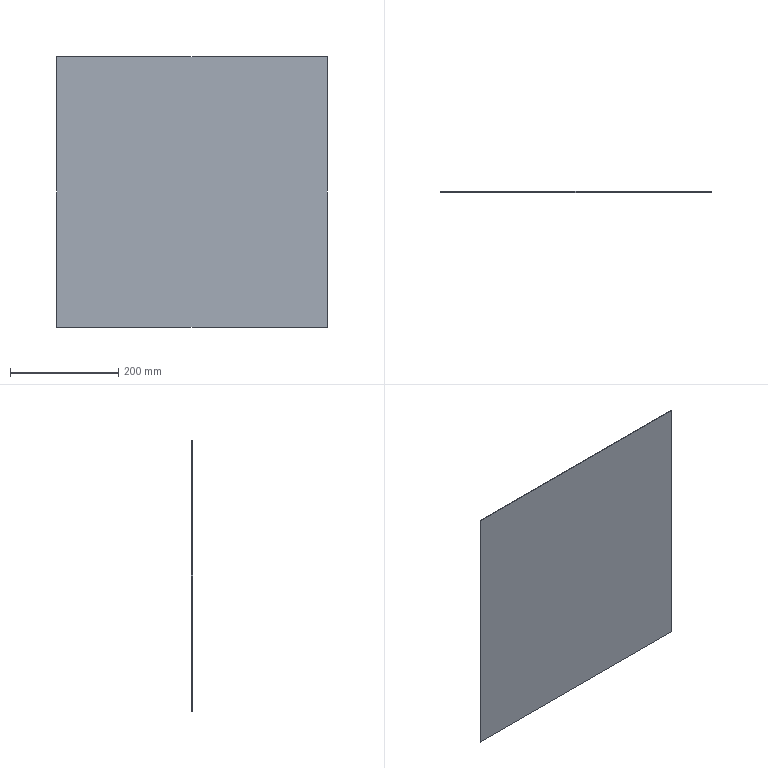Part | STEP file | 1 solid | 6 faces | box 498.959 x 2 x 500 mm | volume 498959 mm3 | plane 6
STEP:
#1=CARTESIAN_POINT('',(0.,0.,0.));
#2=DIRECTION('',(0.,0.,1.));
#3=DIRECTION('',(1.,0.,0.));
#4=AXIS2_PLACEMENT_3D('',#1,#2,#3);
#5=CARTESIAN_POINT('',(600.,-190.836,-106.359));
#6=VERTEX_POINT('',#5);
#7=CARTESIAN_POINT('',(600.,-190.836,393.641));
#8=VERTEX_POINT('',#7);
#9=CARTESIAN_POINT('',(600.,-190.836,-106.359));
#10=DIRECTION('',(0.,0.,1.));
#11=VECTOR('',#10,1.);
#12=LINE('',#9,#11);
#13=CARTESIAN_POINT('',(600.,-188.836,-106.359));
#14=DIRECTION('',(1.,0.,0.));
#15=DIRECTION('',(0.,1.,0.));
#16=AXIS2_PLACEMENT_3D('',#13,#14,#15);
#17=PLANE('',#16);
#18=CARTESIAN_POINT('',(-2.,0.));
#19=DIRECTION('',(0.,1.));
#20=VECTOR('',#19,1.);
#21=LINE('',#18,#20);
#22=(GEOMETRIC_REPRESENTATION_CONTEXT(2)PARAMETRIC_REPRESENTATION_CONTEXT()REPRESENTATION_CONTEXT('',''));
#23=DEFINITIONAL_REPRESENTATION('',(#21),#22);
#24=PCURVE('',#17,#23);
#25=CARTESIAN_POINT('',(0.,-190.836,0.));
#26=DIRECTION('',(0.,1.,0.));
#27=DIRECTION('',(-1.,0.,0.));
#28=AXIS2_PLACEMENT_3D('',#25,#26,#27);
#29=PLANE('',#28);
#30=CARTESIAN_POINT('',(-600.,-106.359));
#31=DIRECTION('',(0.,1.));
#32=VECTOR('',#31,1.);
#33=LINE('',#30,#32);
#34=(GEOMETRIC_REPRESENTATION_CONTEXT(2)PARAMETRIC_REPRESENTATION_CONTEXT()REPRESENTATION_CONTEXT('',''));
#35=DEFINITIONAL_REPRESENTATION('',(#33),#34);
#36=PCURVE('',#29,#35);
#37=SURFACE_CURVE('',#12,(#24,#36),.PCURVE_S1.);
#38=EDGE_CURVE('',#6,#8,#37,.T.);
#39=ORIENTED_EDGE('',*,*,#38,.T.);
#40=CARTESIAN_POINT('',(600.,-188.836,393.641));
#41=VERTEX_POINT('',#40);
#42=CARTESIAN_POINT('',(600.,-188.836,393.641));
#43=DIRECTION('',(0.,-1.,0.));
#44=VECTOR('',#43,1.);
#45=LINE('',#42,#44);
#46=CARTESIAN_POINT('',(0.,500.));
#47=DIRECTION('',(-1.,0.));
#48=VECTOR('',#47,1.);
#49=LINE('',#46,#48);
#50=(GEOMETRIC_REPRESENTATION_CONTEXT(2)PARAMETRIC_REPRESENTATION_CONTEXT()REPRESENTATION_CONTEXT('',''));
#51=DEFINITIONAL_REPRESENTATION('',(#49),#50);
#52=PCURVE('',#17,#51);
#53=CARTESIAN_POINT('',(600.,-188.836,393.641));
#54=DIRECTION('',(0.,0.,-1.));
#55=DIRECTION('',(0.,1.,0.));
#56=AXIS2_PLACEMENT_3D('',#53,#54,#55);
#57=PLANE('',#56);
#58=CARTESIAN_POINT('',(0.,0.));
#59=DIRECTION('',(-1.,0.));
#60=VECTOR('',#59,1.);
#61=LINE('',#58,#60);
#62=(GEOMETRIC_REPRESENTATION_CONTEXT(2)PARAMETRIC_REPRESENTATION_CONTEXT()REPRESENTATION_CONTEXT('',''));
#63=DEFINITIONAL_REPRESENTATION('',(#61),#62);
#64=PCURVE('',#57,#63);
#65=SURFACE_CURVE('',#45,(#52,#64),.PCURVE_S1.);
#66=EDGE_CURVE('',#41,#8,#65,.T.);
#67=ORIENTED_EDGE('',*,*,#66,.F.);
#68=CARTESIAN_POINT('',(600.,-188.836,-106.359));
#69=VERTEX_POINT('',#68);
#70=CARTESIAN_POINT('',(600.,-188.836,-106.359));
#71=DIRECTION('',(0.,0.,1.));
#72=VECTOR('',#71,1.);
#73=LINE('',#70,#72);
#74=CARTESIAN_POINT('',(0.,0.));
#75=DIRECTION('',(0.,1.));
#76=VECTOR('',#75,1.);
#77=LINE('',#74,#76);
#78=(GEOMETRIC_REPRESENTATION_CONTEXT(2)PARAMETRIC_REPRESENTATION_CONTEXT()REPRESENTATION_CONTEXT('',''));
#79=DEFINITIONAL_REPRESENTATION('',(#77),#78);
#80=PCURVE('',#17,#79);
#81=CARTESIAN_POINT('',(0.,-188.836,0.));
#82=DIRECTION('',(0.,1.,0.));
#83=DIRECTION('',(-1.,0.,0.));
#84=AXIS2_PLACEMENT_3D('',#81,#82,#83);
#85=PLANE('',#84);
#86=CARTESIAN_POINT('',(-600.,-106.359));
#87=DIRECTION('',(0.,1.));
#88=VECTOR('',#87,1.);
#89=LINE('',#86,#88);
#90=(GEOMETRIC_REPRESENTATION_CONTEXT(2)PARAMETRIC_REPRESENTATION_CONTEXT()REPRESENTATION_CONTEXT('',''));
#91=DEFINITIONAL_REPRESENTATION('',(#89),#90);
#92=PCURVE('',#85,#91);
#93=SURFACE_CURVE('',#73,(#80,#92),.PCURVE_S1.);
#94=EDGE_CURVE('',#69,#41,#93,.T.);
#95=ORIENTED_EDGE('',*,*,#94,.F.);
#96=CARTESIAN_POINT('',(600.,-188.836,-106.359));
#97=DIRECTION('',(0.,-1.,0.));
#98=VECTOR('',#97,1.);
#99=LINE('',#96,#98);
#100=CARTESIAN_POINT('',(0.,0.));
#101=DIRECTION('',(-1.,0.));
#102=VECTOR('',#101,1.);
#103=LINE('',#100,#102);
#104=(GEOMETRIC_REPRESENTATION_CONTEXT(2)PARAMETRIC_REPRESENTATION_CONTEXT()REPRESENTATION_CONTEXT('',''));
#105=DEFINITIONAL_REPRESENTATION('',(#103),#104);
#106=PCURVE('',#17,#105);
#107=CARTESIAN_POINT('',(600.,-188.836,-106.359));
#108=DIRECTION('',(0.,0.,1.));
#109=DIRECTION('',(0.,-1.,0.));
#110=AXIS2_PLACEMENT_3D('',#107,#108,#109);
#111=PLANE('',#110);
#112=CARTESIAN_POINT('',(0.,0.));
#113=DIRECTION('',(1.,0.));
#114=VECTOR('',#113,1.);
#115=LINE('',#112,#114);
#116=(GEOMETRIC_REPRESENTATION_CONTEXT(2)PARAMETRIC_REPRESENTATION_CONTEXT()REPRESENTATION_CONTEXT('',''));
#117=DEFINITIONAL_REPRESENTATION('',(#115),#116);
#118=PCURVE('',#111,#117);
#119=SURFACE_CURVE('',#99,(#106,#118),.PCURVE_S1.);
#120=EDGE_CURVE('',#69,#6,#119,.T.);
#121=ORIENTED_EDGE('',*,*,#120,.T.);
#122=EDGE_LOOP('',(#39,#67,#95,#121));
#123=FACE_BOUND('',#122,.T.);
#124=ADVANCED_FACE('',(#123),#17,.F.);
#125=CARTESIAN_POINT('',(1098.959,-190.836,393.641));
#126=VERTEX_POINT('',#125);
#127=CARTESIAN_POINT('',(600.,-190.836,393.641));
#128=DIRECTION('',(1.,0.,0.));
#129=VECTOR('',#128,1.);
#130=LINE('',#127,#129);
#131=CARTESIAN_POINT('',(-2.,0.));
#132=DIRECTION('',(0.,1.));
#133=VECTOR('',#132,1.);
#134=LINE('',#131,#133);
#135=(GEOMETRIC_REPRESENTATION_CONTEXT(2)PARAMETRIC_REPRESENTATION_CONTEXT()REPRESENTATION_CONTEXT('',''));
#136=DEFINITIONAL_REPRESENTATION('',(#134),#135);
#137=PCURVE('',#57,#136);
#138=CARTESIAN_POINT('',(-600.,393.641));
#139=DIRECTION('',(-1.,0.));
#140=VECTOR('',#139,1.);
#141=LINE('',#138,#140);
#142=(GEOMETRIC_REPRESENTATION_CONTEXT(2)PARAMETRIC_REPRESENTATION_CONTEXT()REPRESENTATION_CONTEXT('',''));
#143=DEFINITIONAL_REPRESENTATION('',(#141),#142);
#144=PCURVE('',#29,#143);
#145=SURFACE_CURVE('',#130,(#137,#144),.PCURVE_S1.);
#146=EDGE_CURVE('',#8,#126,#145,.T.);
#147=ORIENTED_EDGE('',*,*,#146,.T.);
#148=CARTESIAN_POINT('',(1098.959,-188.836,393.641));
#149=VERTEX_POINT('',#148);
#150=CARTESIAN_POINT('',(1098.959,-188.836,393.641));
#151=DIRECTION('',(0.,-1.,0.));
#152=VECTOR('',#151,1.);
#153=LINE('',#150,#152);
#154=CARTESIAN_POINT('',(0.,498.959));
#155=DIRECTION('',(-1.,0.));
#156=VECTOR('',#155,1.);
#157=LINE('',#154,#156);
#158=(GEOMETRIC_REPRESENTATION_CONTEXT(2)PARAMETRIC_REPRESENTATION_CONTEXT()REPRESENTATION_CONTEXT('',''));
#159=DEFINITIONAL_REPRESENTATION('',(#157),#158);
#160=PCURVE('',#57,#159);
#161=CARTESIAN_POINT('',(1098.959,-188.836,-106.359));
#162=DIRECTION('',(-1.,0.,0.));
#163=DIRECTION('',(0.,-1.,0.));
#164=AXIS2_PLACEMENT_3D('',#161,#162,#163);
#165=PLANE('',#164);
#166=CARTESIAN_POINT('',(0.,500.));
#167=DIRECTION('',(1.,0.));
#168=VECTOR('',#167,1.);
#169=LINE('',#166,#168);
#170=(GEOMETRIC_REPRESENTATION_CONTEXT(2)PARAMETRIC_REPRESENTATION_CONTEXT()REPRESENTATION_CONTEXT('',''));
#171=DEFINITIONAL_REPRESENTATION('',(#169),#170);
#172=PCURVE('',#165,#171);
#173=SURFACE_CURVE('',#153,(#160,#172),.PCURVE_S1.);
#174=EDGE_CURVE('',#149,#126,#173,.T.);
#175=ORIENTED_EDGE('',*,*,#174,.F.);
#176=CARTESIAN_POINT('',(600.,-188.836,393.641));
#177=DIRECTION('',(1.,0.,0.));
#178=VECTOR('',#177,1.);
#179=LINE('',#176,#178);
#180=CARTESIAN_POINT('',(0.,0.));
#181=DIRECTION('',(0.,1.));
#182=VECTOR('',#181,1.);
#183=LINE('',#180,#182);
#184=(GEOMETRIC_REPRESENTATION_CONTEXT(2)PARAMETRIC_REPRESENTATION_CONTEXT()REPRESENTATION_CONTEXT('',''));
#185=DEFINITIONAL_REPRESENTATION('',(#183),#184);
#186=PCURVE('',#57,#185);
#187=CARTESIAN_POINT('',(-600.,393.641));
#188=DIRECTION('',(-1.,0.));
#189=VECTOR('',#188,1.);
#190=LINE('',#187,#189);
#191=(GEOMETRIC_REPRESENTATION_CONTEXT(2)PARAMETRIC_REPRESENTATION_CONTEXT()REPRESENTATION_CONTEXT('',''));
#192=DEFINITIONAL_REPRESENTATION('',(#190),#191);
#193=PCURVE('',#85,#192);
#194=SURFACE_CURVE('',#179,(#186,#193),.PCURVE_S1.);
#195=EDGE_CURVE('',#41,#149,#194,.T.);
#196=ORIENTED_EDGE('',*,*,#195,.F.);
#197=ORIENTED_EDGE('',*,*,#66,.T.);
#198=EDGE_LOOP('',(#147,#175,#196,#197));
#199=FACE_BOUND('',#198,.T.);
#200=ADVANCED_FACE('',(#199),#57,.F.);
#201=CARTESIAN_POINT('',(1098.959,-190.836,-106.359));
#202=VERTEX_POINT('',#201);
#203=CARTESIAN_POINT('',(1098.959,-190.836,-106.359));
#204=DIRECTION('',(0.,0.,-1.));
#205=VECTOR('',#204,1.);
#206=LINE('',#203,#205);
#207=CARTESIAN_POINT('',(2.,0.));
#208=DIRECTION('',(0.,-1.));
#209=VECTOR('',#208,1.);
#210=LINE('',#207,#209);
#211=(GEOMETRIC_REPRESENTATION_CONTEXT(2)PARAMETRIC_REPRESENTATION_CONTEXT()REPRESENTATION_CONTEXT('',''));
#212=DEFINITIONAL_REPRESENTATION('',(#210),#211);
#213=PCURVE('',#165,#212);
#214=CARTESIAN_POINT('',(-1098.959,-106.359));
#215=DIRECTION('',(0.,-1.));
#216=VECTOR('',#215,1.);
#217=LINE('',#214,#216);
#218=(GEOMETRIC_REPRESENTATION_CONTEXT(2)PARAMETRIC_REPRESENTATION_CONTEXT()REPRESENTATION_CONTEXT('',''));
#219=DEFINITIONAL_REPRESENTATION('',(#217),#218);
#220=PCURVE('',#29,#219);
#221=SURFACE_CURVE('',#206,(#213,#220),.PCURVE_S1.);
#222=EDGE_CURVE('',#126,#202,#221,.T.);
#223=ORIENTED_EDGE('',*,*,#222,.T.);
#224=CARTESIAN_POINT('',(1098.959,-188.836,-106.359));
#225=VERTEX_POINT('',#224);
#226=CARTESIAN_POINT('',(1098.959,-188.836,-106.359));
#227=DIRECTION('',(0.,-1.,0.));
#228=VECTOR('',#227,1.);
#229=LINE('',#226,#228);
#230=CARTESIAN_POINT('',(0.,0.));
#231=DIRECTION('',(1.,0.));
#232=VECTOR('',#231,1.);
#233=LINE('',#230,#232);
#234=(GEOMETRIC_REPRESENTATION_CONTEXT(2)PARAMETRIC_REPRESENTATION_CONTEXT()REPRESENTATION_CONTEXT('',''));
#235=DEFINITIONAL_REPRESENTATION('',(#233),#234);
#236=PCURVE('',#165,#235);
#237=CARTESIAN_POINT('',(0.,498.959));
#238=DIRECTION('',(1.,0.));
#239=VECTOR('',#238,1.);
#240=LINE('',#237,#239);
#241=(GEOMETRIC_REPRESENTATION_CONTEXT(2)PARAMETRIC_REPRESENTATION_CONTEXT()REPRESENTATION_CONTEXT('',''));
#242=DEFINITIONAL_REPRESENTATION('',(#240),#241);
#243=PCURVE('',#111,#242);
#244=SURFACE_CURVE('',#229,(#236,#243),.PCURVE_S1.);
#245=EDGE_CURVE('',#225,#202,#244,.T.);
#246=ORIENTED_EDGE('',*,*,#245,.F.);
#247=CARTESIAN_POINT('',(1098.959,-188.836,-106.359));
#248=DIRECTION('',(0.,0.,-1.));
#249=VECTOR('',#248,1.);
#250=LINE('',#247,#249);
#251=CARTESIAN_POINT('',(0.,0.));
#252=DIRECTION('',(0.,-1.));
#253=VECTOR('',#252,1.);
#254=LINE('',#251,#253);
#255=(GEOMETRIC_REPRESENTATION_CONTEXT(2)PARAMETRIC_REPRESENTATION_CONTEXT()REPRESENTATION_CONTEXT('',''));
#256=DEFINITIONAL_REPRESENTATION('',(#254),#255);
#257=PCURVE('',#165,#256);
#258=CARTESIAN_POINT('',(-1098.959,-106.359));
#259=DIRECTION('',(0.,-1.));
#260=VECTOR('',#259,1.);
#261=LINE('',#258,#260);
#262=(GEOMETRIC_REPRESENTATION_CONTEXT(2)PARAMETRIC_REPRESENTATION_CONTEXT()REPRESENTATION_CONTEXT('',''));
#263=DEFINITIONAL_REPRESENTATION('',(#261),#262);
#264=PCURVE('',#85,#263);
#265=SURFACE_CURVE('',#250,(#257,#264),.PCURVE_S1.);
#266=EDGE_CURVE('',#149,#225,#265,.T.);
#267=ORIENTED_EDGE('',*,*,#266,.F.);
#268=ORIENTED_EDGE('',*,*,#174,.T.);
#269=EDGE_LOOP('',(#223,#246,#267,#268));
#270=FACE_BOUND('',#269,.T.);
#271=ADVANCED_FACE('',(#270),#165,.F.);
#272=CARTESIAN_POINT('',(600.,-190.836,-106.359));
#273=DIRECTION('',(-1.,0.,0.));
#274=VECTOR('',#273,1.);
#275=LINE('',#272,#274);
#276=CARTESIAN_POINT('',(2.,0.));
#277=DIRECTION('',(0.,-1.));
#278=VECTOR('',#277,1.);
#279=LINE('',#276,#278);
#280=(GEOMETRIC_REPRESENTATION_CONTEXT(2)PARAMETRIC_REPRESENTATION_CONTEXT()REPRESENTATION_CONTEXT('',''));
#281=DEFINITIONAL_REPRESENTATION('',(#279),#280);
#282=PCURVE('',#111,#281);
#283=CARTESIAN_POINT('',(-600.,-106.359));
#284=DIRECTION('',(1.,0.));
#285=VECTOR('',#284,1.);
#286=LINE('',#283,#285);
#287=(GEOMETRIC_REPRESENTATION_CONTEXT(2)PARAMETRIC_REPRESENTATION_CONTEXT()REPRESENTATION_CONTEXT('',''));
#288=DEFINITIONAL_REPRESENTATION('',(#286),#287);
#289=PCURVE('',#29,#288);
#290=SURFACE_CURVE('',#275,(#282,#289),.PCURVE_S1.);
#291=EDGE_CURVE('',#202,#6,#290,.T.);
#292=ORIENTED_EDGE('',*,*,#291,.T.);
#293=ORIENTED_EDGE('',*,*,#120,.F.);
#294=CARTESIAN_POINT('',(600.,-188.836,-106.359));
#295=DIRECTION('',(-1.,0.,0.));
#296=VECTOR('',#295,1.);
#297=LINE('',#294,#296);
#298=CARTESIAN_POINT('',(0.,0.));
#299=DIRECTION('',(0.,-1.));
#300=VECTOR('',#299,1.);
#301=LINE('',#298,#300);
#302=(GEOMETRIC_REPRESENTATION_CONTEXT(2)PARAMETRIC_REPRESENTATION_CONTEXT()REPRESENTATION_CONTEXT('',''));
#303=DEFINITIONAL_REPRESENTATION('',(#301),#302);
#304=PCURVE('',#111,#303);
#305=CARTESIAN_POINT('',(-600.,-106.359));
#306=DIRECTION('',(1.,0.));
#307=VECTOR('',#306,1.);
#308=LINE('',#305,#307);
#309=(GEOMETRIC_REPRESENTATION_CONTEXT(2)PARAMETRIC_REPRESENTATION_CONTEXT()REPRESENTATION_CONTEXT('',''));
#310=DEFINITIONAL_REPRESENTATION('',(#308),#309);
#311=PCURVE('',#85,#310);
#312=SURFACE_CURVE('',#297,(#304,#311),.PCURVE_S1.);
#313=EDGE_CURVE('',#225,#69,#312,.T.);
#314=ORIENTED_EDGE('',*,*,#313,.F.);
#315=ORIENTED_EDGE('',*,*,#245,.T.);
#316=EDGE_LOOP('',(#292,#293,#314,#315));
#317=FACE_BOUND('',#316,.T.);
#318=ADVANCED_FACE('',(#317),#111,.F.);
#319=ORIENTED_EDGE('',*,*,#94,.T.);
#320=ORIENTED_EDGE('',*,*,#195,.T.);
#321=ORIENTED_EDGE('',*,*,#266,.T.);
#322=ORIENTED_EDGE('',*,*,#313,.T.);
#323=EDGE_LOOP('',(#319,#320,#321,#322));
#324=FACE_BOUND('',#323,.T.);
#325=ADVANCED_FACE('',(#324),#85,.T.);
#326=ORIENTED_EDGE('',*,*,#38,.F.);
#327=ORIENTED_EDGE('',*,*,#291,.F.);
#328=ORIENTED_EDGE('',*,*,#222,.F.);
#329=ORIENTED_EDGE('',*,*,#146,.F.);
#330=EDGE_LOOP('',(#326,#327,#328,#329));
#331=FACE_BOUND('',#330,.T.);
#332=ADVANCED_FACE('',(#331),#29,.F.);
#333=CLOSED_SHELL('',(#124,#200,#271,#318,#325,#332));
#334=MANIFOLD_SOLID_BREP('',#333);
#335=(LENGTH_UNIT()NAMED_UNIT(*)SI_UNIT(.MILLI.,.METRE.));
#336=UNCERTAINTY_MEASURE_WITH_UNIT(LENGTH_MEASURE(0.0000001),#335,'','');
#337=(NAMED_UNIT(*)PLANE_ANGLE_UNIT()SI_UNIT($,.RADIAN.));
#338=(NAMED_UNIT(*)SI_UNIT($,.STERADIAN.)SOLID_ANGLE_UNIT());
#339=(GEOMETRIC_REPRESENTATION_CONTEXT(3)GLOBAL_UNCERTAINTY_ASSIGNED_CONTEXT((#336))GLOBAL_UNIT_ASSIGNED_CONTEXT((#335,#337,#338))REPRESENTATION_CONTEXT('',''));
#340=ADVANCED_BREP_SHAPE_REPRESENTATION('',(#4,#334),#339);